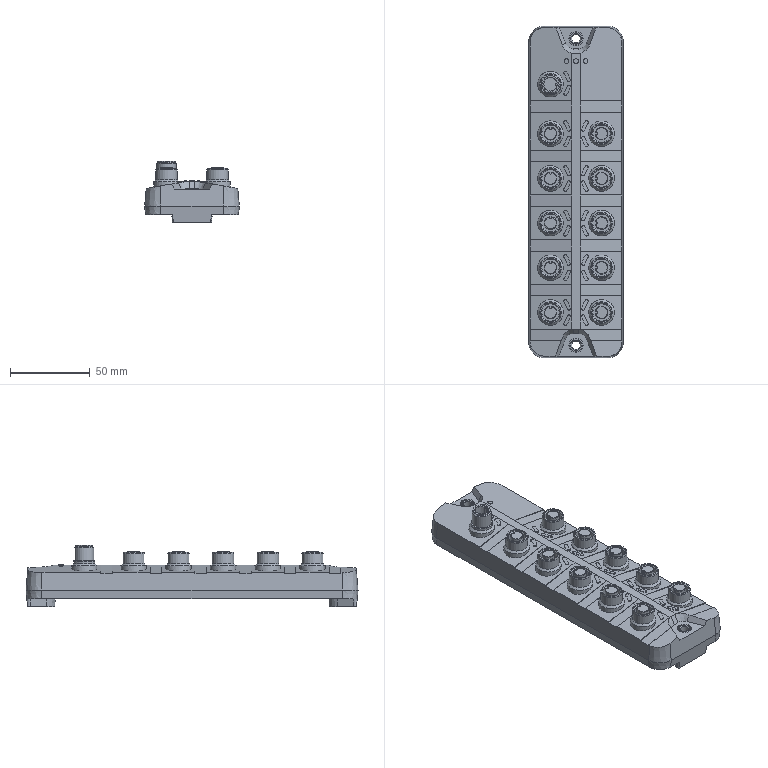Part | NX | features BREP 1 | 1 solid | 415 faces | box 59.3 x 208 x 38.25 mm | volume 240538 mm3 | plane 178 | cylinder 169 | cone 58 | torus 10 | commonest cylinder face diameters 2 x44 21.4 x22 25.4 x22 1.2 x21 13.5 x11 16 x11